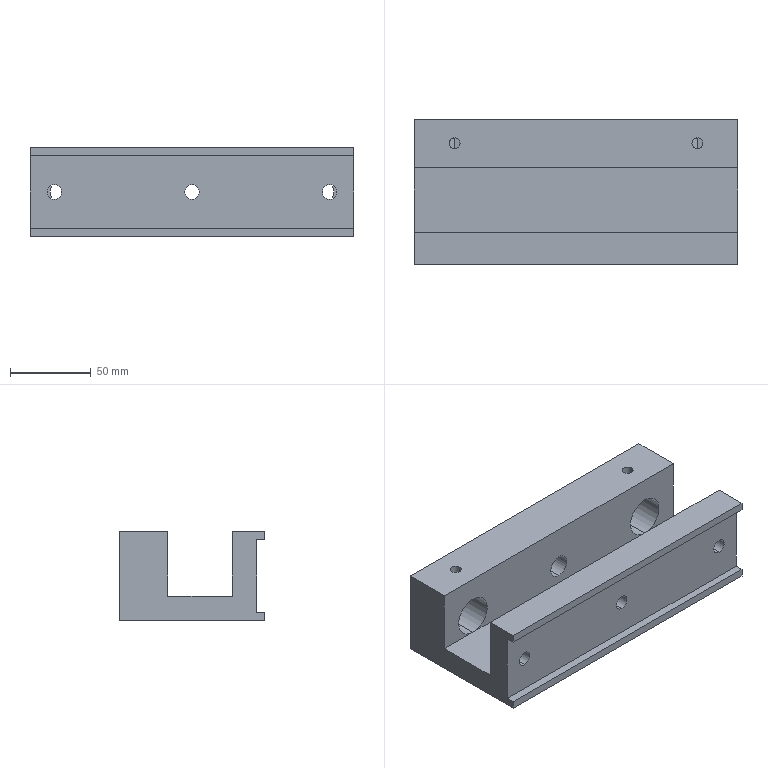Part | STEP file | BCC3 H13_2 | 1 solid | 30 faces | box 200 x 90 x 55 mm | volume 586969 mm3 | cylinder 16 | plane 14 | commonest cylinder face diameters 9 x6 6.8 x4 25 x4 14 x2